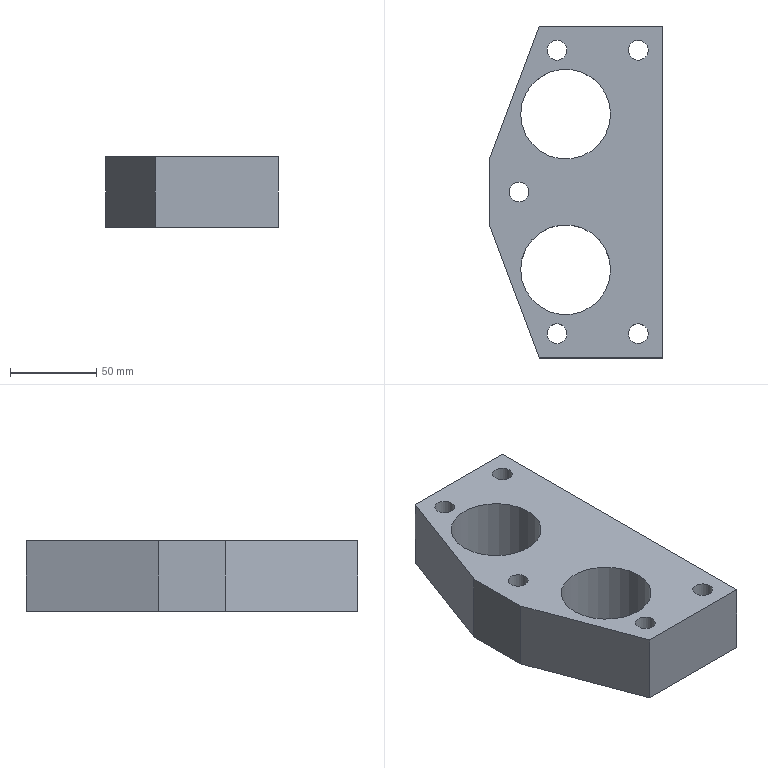Part | NX | features solid 2 | 1 solid | 25 faces | box 100 x 192 x 41 mm | volume 491723 mm3 | plane 13 | cylinder 12 | commonest cylinder face diameters 11.5 x5 18 x5 52 x2
STEP:
#1=CARTESIAN_POINT('',(1356.,82.,60.));
#2=VERTEX_POINT('',#1);
#3=CARTESIAN_POINT('',(1347.,82.,60.));
#4=DIRECTION('',(0.,0.,1.));
#5=DIRECTION('',(1.,0.,0.));
#6=AXIS2_PLACEMENT_3D('',#3,#4,#5);
#7=CIRCLE('',#6,9.);
#8=EDGE_CURVE('',#2,#2,#7,.T.);
#9=ORIENTED_EDGE('',*,*,#8,.T.);
#10=EDGE_LOOP('',(#9));
#11=FACE_BOUND('',#10,.T.);
#12=CARTESIAN_POINT('',(1287.,0.,60.));
#13=VERTEX_POINT('',#12);
#14=CARTESIAN_POINT('',(1278.,0.,60.));
#15=DIRECTION('',(0.,0.,1.));
#16=DIRECTION('',(1.,0.,0.));
#17=AXIS2_PLACEMENT_3D('',#14,#15,#16);
#18=CIRCLE('',#17,9.);
#19=EDGE_CURVE('',#13,#13,#18,.T.);
#20=ORIENTED_EDGE('',*,*,#19,.T.);
#21=EDGE_LOOP('',(#20));
#22=FACE_BOUND('',#21,.T.);
#23=CARTESIAN_POINT('',(1356.,-82.,60.));
#24=VERTEX_POINT('',#23);
#25=CARTESIAN_POINT('',(1347.,-82.,60.));
#26=DIRECTION('',(0.,0.,1.));
#27=DIRECTION('',(1.,0.,0.));
#28=AXIS2_PLACEMENT_3D('',#25,#26,#27);
#29=CIRCLE('',#28,9.);
#30=EDGE_CURVE('',#24,#24,#29,.T.);
#31=ORIENTED_EDGE('',*,*,#30,.T.);
#32=EDGE_LOOP('',(#31));
#33=FACE_BOUND('',#32,.T.);
#34=CARTESIAN_POINT('',(1261.,19.27,60.));
#35=VERTEX_POINT('',#34);
#36=CARTESIAN_POINT('',(1261.,-19.27,60.));
#37=VERTEX_POINT('',#36);
#38=CARTESIAN_POINT('',(1261.,0.,60.));
#39=DIRECTION('',(0.,-1.,0.));
#40=VECTOR('',#39,1000.);
#41=LINE('',#38,#40);
#42=EDGE_CURVE('',#35,#37,#41,.T.);
#43=ORIENTED_EDGE('',*,*,#42,.F.);
#44=CARTESIAN_POINT('',(1289.688,96.,60.));
#45=VERTEX_POINT('',#44);
#46=CARTESIAN_POINT('',(1383.637,347.282,60.));
#47=DIRECTION('',(-0.3502,-0.9367,0.));
#48=VECTOR('',#47,1000.);
#49=LINE('',#46,#48);
#50=EDGE_CURVE('',#45,#35,#49,.T.);
#51=ORIENTED_EDGE('',*,*,#50,.F.);
#52=CARTESIAN_POINT('',(1361.,96.,60.));
#53=VERTEX_POINT('',#52);
#54=CARTESIAN_POINT('',(1390.,96.,60.));
#55=DIRECTION('',(1.,0.,0.));
#56=VECTOR('',#55,1000.);
#57=LINE('',#54,#56);
#58=EDGE_CURVE('',#45,#53,#57,.T.);
#59=ORIENTED_EDGE('',*,*,#58,.T.);
#60=CARTESIAN_POINT('',(1361.,-96.,60.));
#61=VERTEX_POINT('',#60);
#62=CARTESIAN_POINT('',(1361.,0.,60.));
#63=DIRECTION('',(0.,1.,0.));
#64=VECTOR('',#63,1000.);
#65=LINE('',#62,#64);
#66=EDGE_CURVE('',#61,#53,#65,.T.);
#67=ORIENTED_EDGE('',*,*,#66,.F.);
#68=CARTESIAN_POINT('',(1289.688,-96.,60.));
#69=VERTEX_POINT('',#68);
#70=CARTESIAN_POINT('',(1390.,-96.,60.));
#71=DIRECTION('',(1.,0.,0.));
#72=VECTOR('',#71,1000.);
#73=LINE('',#70,#72);
#74=EDGE_CURVE('',#69,#61,#73,.T.);
#75=ORIENTED_EDGE('',*,*,#74,.F.);
#76=CARTESIAN_POINT('',(1383.637,-347.282,60.));
#77=DIRECTION('',(-0.3502,0.9367,0.));
#78=VECTOR('',#77,1000.);
#79=LINE('',#76,#78);
#80=EDGE_CURVE('',#69,#37,#79,.T.);
#81=ORIENTED_EDGE('',*,*,#80,.T.);
#82=EDGE_LOOP('',(#43,#51,#59,#67,#75,#81));
#83=FACE_BOUND('',#82,.T.);
#84=CARTESIAN_POINT('',(1309.,-82.,60.));
#85=VERTEX_POINT('',#84);
#86=CARTESIAN_POINT('',(1300.,-82.,60.));
#87=DIRECTION('',(0.,0.,1.));
#88=DIRECTION('',(1.,0.,0.));
#89=AXIS2_PLACEMENT_3D('',#86,#87,#88);
#90=CIRCLE('',#89,9.);
#91=EDGE_CURVE('',#85,#85,#90,.T.);
#92=ORIENTED_EDGE('',*,*,#91,.T.);
#93=EDGE_LOOP('',(#92));
#94=FACE_BOUND('',#93,.T.);
#95=CARTESIAN_POINT('',(1309.,82.,60.));
#96=VERTEX_POINT('',#95);
#97=CARTESIAN_POINT('',(1300.,82.,60.));
#98=DIRECTION('',(0.,0.,1.));
#99=DIRECTION('',(1.,0.,0.));
#100=AXIS2_PLACEMENT_3D('',#97,#98,#99);
#101=CIRCLE('',#100,9.);
#102=EDGE_CURVE('',#96,#96,#101,.T.);
#103=ORIENTED_EDGE('',*,*,#102,.T.);
#104=EDGE_LOOP('',(#103));
#105=FACE_BOUND('',#104,.T.);
#106=CARTESIAN_POINT('',(1331.,-45.,60.));
#107=VERTEX_POINT('',#106);
#108=CARTESIAN_POINT('',(1305.,-45.,60.));
#109=DIRECTION('',(0.,0.,1.));
#110=DIRECTION('',(1.,0.,0.));
#111=AXIS2_PLACEMENT_3D('',#108,#109,#110);
#112=CIRCLE('',#111,26.);
#113=EDGE_CURVE('',#107,#107,#112,.T.);
#114=ORIENTED_EDGE('',*,*,#113,.T.);
#115=EDGE_LOOP('',(#114));
#116=FACE_BOUND('',#115,.T.);
#117=CARTESIAN_POINT('',(1331.,45.,60.));
#118=VERTEX_POINT('',#117);
#119=CARTESIAN_POINT('',(1305.,45.,60.));
#120=DIRECTION('',(0.,0.,1.));
#121=DIRECTION('',(1.,0.,0.));
#122=AXIS2_PLACEMENT_3D('',#119,#120,#121);
#123=CIRCLE('',#122,26.);
#124=EDGE_CURVE('',#118,#118,#123,.T.);
#125=ORIENTED_EDGE('',*,*,#124,.T.);
#126=EDGE_LOOP('',(#125));
#127=FACE_BOUND('',#126,.T.);
#128=CARTESIAN_POINT('',(2312.5,0.,60.));
#129=DIRECTION('',(0.,0.,1.));
#130=DIRECTION('',(-1.,0.,0.));
#131=AXIS2_PLACEMENT_3D('',#128,#129,#130);
#132=PLANE('',#131);
#133=ADVANCED_FACE('',(#11,#22,#33,#83,#94,#105,#116,#127),#132,.F.);
#134=CARTESIAN_POINT('',(1361.,96.,101.));
#135=VERTEX_POINT('',#134);
#136=CARTESIAN_POINT('',(1361.,-96.,101.));
#137=VERTEX_POINT('',#136);
#138=CARTESIAN_POINT('',(1361.,0.,101.));
#139=DIRECTION('',(0.,-1.,0.));
#140=VECTOR('',#139,1000.);
#141=LINE('',#138,#140);
#142=EDGE_CURVE('',#135,#137,#141,.T.);
#143=ORIENTED_EDGE('',*,*,#142,.F.);
#144=CARTESIAN_POINT('',(1289.688,96.,101.));
#145=VERTEX_POINT('',#144);
#146=CARTESIAN_POINT('',(1390.,96.,101.));
#147=DIRECTION('',(-1.,0.,0.));
#148=VECTOR('',#147,1000.);
#149=LINE('',#146,#148);
#150=EDGE_CURVE('',#135,#145,#149,.T.);
#151=ORIENTED_EDGE('',*,*,#150,.T.);
#152=CARTESIAN_POINT('',(1261.,19.27,101.));
#153=VERTEX_POINT('',#152);
#154=CARTESIAN_POINT('',(1071.365,-487.94,101.));
#155=DIRECTION('',(0.3502,0.9367,0.));
#156=VECTOR('',#155,1000.);
#157=LINE('',#154,#156);
#158=EDGE_CURVE('',#153,#145,#157,.T.);
#159=ORIENTED_EDGE('',*,*,#158,.F.);
#160=CARTESIAN_POINT('',(1261.,-19.27,101.));
#161=VERTEX_POINT('',#160);
#162=CARTESIAN_POINT('',(1261.,0.,101.));
#163=DIRECTION('',(0.,1.,0.));
#164=VECTOR('',#163,1000.);
#165=LINE('',#162,#164);
#166=EDGE_CURVE('',#161,#153,#165,.T.);
#167=ORIENTED_EDGE('',*,*,#166,.F.);
#168=CARTESIAN_POINT('',(1289.688,-96.,101.));
#169=VERTEX_POINT('',#168);
#170=CARTESIAN_POINT('',(1071.365,487.94,101.));
#171=DIRECTION('',(0.3502,-0.9367,0.));
#172=VECTOR('',#171,1000.);
#173=LINE('',#170,#172);
#174=EDGE_CURVE('',#161,#169,#173,.T.);
#175=ORIENTED_EDGE('',*,*,#174,.T.);
#176=CARTESIAN_POINT('',(1390.,-96.,101.));
#177=DIRECTION('',(-1.,0.,0.));
#178=VECTOR('',#177,1000.);
#179=LINE('',#176,#178);
#180=EDGE_CURVE('',#137,#169,#179,.T.);
#181=ORIENTED_EDGE('',*,*,#180,.F.);
#182=EDGE_LOOP('',(#143,#151,#159,#167,#175,#181));
#183=FACE_BOUND('',#182,.T.);
#184=CARTESIAN_POINT('',(1352.75,-82.,101.));
#185=VERTEX_POINT('',#184);
#186=CARTESIAN_POINT('',(1347.,-82.,101.));
#187=DIRECTION('',(0.,0.,1.));
#188=DIRECTION('',(1.,0.,0.));
#189=AXIS2_PLACEMENT_3D('',#186,#187,#188);
#190=CIRCLE('',#189,5.75);
#191=EDGE_CURVE('',#185,#185,#190,.T.);
#192=ORIENTED_EDGE('',*,*,#191,.F.);
#193=EDGE_LOOP('',(#192));
#194=FACE_BOUND('',#193,.T.);
#195=CARTESIAN_POINT('',(1305.75,-82.,101.));
#196=VERTEX_POINT('',#195);
#197=CARTESIAN_POINT('',(1300.,-82.,101.));
#198=DIRECTION('',(0.,0.,1.));
#199=DIRECTION('',(1.,0.,0.));
#200=AXIS2_PLACEMENT_3D('',#197,#198,#199);
#201=CIRCLE('',#200,5.75);
#202=EDGE_CURVE('',#196,#196,#201,.T.);
#203=ORIENTED_EDGE('',*,*,#202,.F.);
#204=EDGE_LOOP('',(#203));
#205=FACE_BOUND('',#204,.T.);
#206=CARTESIAN_POINT('',(1283.75,0.,101.));
#207=VERTEX_POINT('',#206);
#208=CARTESIAN_POINT('',(1278.,0.,101.));
#209=DIRECTION('',(0.,0.,1.));
#210=DIRECTION('',(1.,0.,0.));
#211=AXIS2_PLACEMENT_3D('',#208,#209,#210);
#212=CIRCLE('',#211,5.75);
#213=EDGE_CURVE('',#207,#207,#212,.T.);
#214=ORIENTED_EDGE('',*,*,#213,.F.);
#215=EDGE_LOOP('',(#214));
#216=FACE_BOUND('',#215,.T.);
#217=CARTESIAN_POINT('',(1305.75,82.,101.));
#218=VERTEX_POINT('',#217);
#219=CARTESIAN_POINT('',(1300.,82.,101.));
#220=DIRECTION('',(0.,0.,1.));
#221=DIRECTION('',(1.,0.,0.));
#222=AXIS2_PLACEMENT_3D('',#219,#220,#221);
#223=CIRCLE('',#222,5.75);
#224=EDGE_CURVE('',#218,#218,#223,.T.);
#225=ORIENTED_EDGE('',*,*,#224,.F.);
#226=EDGE_LOOP('',(#225));
#227=FACE_BOUND('',#226,.T.);
#228=CARTESIAN_POINT('',(1352.75,82.,101.));
#229=VERTEX_POINT('',#228);
#230=CARTESIAN_POINT('',(1347.,82.,101.));
#231=DIRECTION('',(0.,0.,1.));
#232=DIRECTION('',(1.,0.,0.));
#233=AXIS2_PLACEMENT_3D('',#230,#231,#232);
#234=CIRCLE('',#233,5.75);
#235=EDGE_CURVE('',#229,#229,#234,.T.);
#236=ORIENTED_EDGE('',*,*,#235,.F.);
#237=EDGE_LOOP('',(#236));
#238=FACE_BOUND('',#237,.T.);
#239=CARTESIAN_POINT('',(1331.,-45.,101.));
#240=VERTEX_POINT('',#239);
#241=CARTESIAN_POINT('',(1305.,-45.,101.));
#242=DIRECTION('',(0.,0.,-1.));
#243=DIRECTION('',(1.,0.,0.));
#244=AXIS2_PLACEMENT_3D('',#241,#242,#243);
#245=CIRCLE('',#244,26.);
#246=EDGE_CURVE('',#240,#240,#245,.T.);
#247=ORIENTED_EDGE('',*,*,#246,.T.);
#248=EDGE_LOOP('',(#247));
#249=FACE_BOUND('',#248,.T.);
#250=CARTESIAN_POINT('',(1331.,45.,101.));
#251=VERTEX_POINT('',#250);
#252=CARTESIAN_POINT('',(1305.,45.,101.));
#253=DIRECTION('',(0.,0.,1.));
#254=DIRECTION('',(1.,0.,0.));
#255=AXIS2_PLACEMENT_3D('',#252,#253,#254);
#256=CIRCLE('',#255,26.);
#257=EDGE_CURVE('',#251,#251,#256,.T.);
#258=ORIENTED_EDGE('',*,*,#257,.F.);
#259=EDGE_LOOP('',(#258));
#260=FACE_BOUND('',#259,.T.);
#261=CARTESIAN_POINT('',(282.5,193.,101.));
#262=DIRECTION('',(0.,0.,1.));
#263=DIRECTION('',(-1.,0.,0.));
#264=AXIS2_PLACEMENT_3D('',#261,#262,#263);
#265=PLANE('',#264);
#266=ADVANCED_FACE('',(#183,#194,#205,#216,#227,#238,#249,#260),#265,.T.);
#267=ORIENTED_EDGE('',*,*,#166,.T.);
#268=CARTESIAN_POINT('',(1261.,19.27,-25.));
#269=DIRECTION('',(0.,0.,1.));
#270=VECTOR('',#269,1000.);
#271=LINE('',#268,#270);
#272=EDGE_CURVE('',#35,#153,#271,.T.);
#273=ORIENTED_EDGE('',*,*,#272,.F.);
#274=ORIENTED_EDGE('',*,*,#42,.T.);
#275=CARTESIAN_POINT('',(1261.,-19.27,-25.));
#276=DIRECTION('',(0.,0.,1.));
#277=VECTOR('',#276,1000.);
#278=LINE('',#275,#277);
#279=EDGE_CURVE('',#37,#161,#278,.T.);
#280=ORIENTED_EDGE('',*,*,#279,.T.);
#281=EDGE_LOOP('',(#267,#273,#274,#280));
#282=FACE_BOUND('',#281,.T.);
#283=CARTESIAN_POINT('',(1261.,0.,-25.));
#284=DIRECTION('',(-1.,0.,0.));
#285=DIRECTION('',(0.,0.,-1.));
#286=AXIS2_PLACEMENT_3D('',#283,#284,#285);
#287=PLANE('',#286);
#288=ADVANCED_FACE('',(#282),#287,.T.);
#289=ORIENTED_EDGE('',*,*,#66,.T.);
#290=CARTESIAN_POINT('',(1361.,96.,0.));
#291=DIRECTION('',(0.,0.,1.));
#292=VECTOR('',#291,1000.);
#293=LINE('',#290,#292);
#294=EDGE_CURVE('',#53,#135,#293,.T.);
#295=ORIENTED_EDGE('',*,*,#294,.T.);
#296=ORIENTED_EDGE('',*,*,#142,.T.);
#297=CARTESIAN_POINT('',(1361.,-96.,0.));
#298=DIRECTION('',(0.,0.,1.));
#299=VECTOR('',#298,1000.);
#300=LINE('',#297,#299);
#301=EDGE_CURVE('',#61,#137,#300,.T.);
#302=ORIENTED_EDGE('',*,*,#301,.F.);
#303=EDGE_LOOP('',(#289,#295,#296,#302));
#304=FACE_BOUND('',#303,.T.);
#305=CARTESIAN_POINT('',(1361.,0.,-25.));
#306=DIRECTION('',(1.,0.,0.));
#307=DIRECTION('',(0.,0.,1.));
#308=AXIS2_PLACEMENT_3D('',#305,#306,#307);
#309=PLANE('',#308);
#310=ADVANCED_FACE('',(#304),#309,.T.);
#311=ORIENTED_EDGE('',*,*,#180,.T.);
#312=CARTESIAN_POINT('',(1289.688,-96.,0.));
#313=DIRECTION('',(0.,0.,-1.));
#314=VECTOR('',#313,1000.);
#315=LINE('',#312,#314);
#316=EDGE_CURVE('',#169,#69,#315,.T.);
#317=ORIENTED_EDGE('',*,*,#316,.T.);
#318=ORIENTED_EDGE('',*,*,#74,.T.);
#319=ORIENTED_EDGE('',*,*,#301,.T.);
#320=EDGE_LOOP('',(#311,#317,#318,#319));
#321=FACE_BOUND('',#320,.T.);
#322=CARTESIAN_POINT('',(1390.,-96.,0.));
#323=DIRECTION('',(0.,-1.,0.));
#324=DIRECTION('',(0.,0.,1.));
#325=AXIS2_PLACEMENT_3D('',#322,#323,#324);
#326=PLANE('',#325);
#327=ADVANCED_FACE('',(#321),#326,.T.);
#328=ORIENTED_EDGE('',*,*,#174,.F.);
#329=ORIENTED_EDGE('',*,*,#279,.F.);
#330=ORIENTED_EDGE('',*,*,#80,.F.);
#331=ORIENTED_EDGE('',*,*,#316,.F.);
#332=EDGE_LOOP('',(#328,#329,#330,#331));
#333=FACE_BOUND('',#332,.T.);
#334=CARTESIAN_POINT('',(1289.418,-95.278,-40.));
#335=DIRECTION('',(-0.9367,-0.3502,0.));
#336=DIRECTION('',(0.3502,-0.9367,0.));
#337=AXIS2_PLACEMENT_3D('',#334,#335,#336);
#338=PLANE('',#337);
#339=ADVANCED_FACE('',(#333),#338,.T.);
#340=ORIENTED_EDGE('',*,*,#150,.F.);
#341=ORIENTED_EDGE('',*,*,#294,.F.);
#342=ORIENTED_EDGE('',*,*,#58,.F.);
#343=CARTESIAN_POINT('',(1289.688,96.,0.));
#344=DIRECTION('',(0.,0.,-1.));
#345=VECTOR('',#344,1000.);
#346=LINE('',#343,#345);
#347=EDGE_CURVE('',#145,#45,#346,.T.);
#348=ORIENTED_EDGE('',*,*,#347,.F.);
#349=EDGE_LOOP('',(#340,#341,#342,#348));
#350=FACE_BOUND('',#349,.T.);
#351=CARTESIAN_POINT('',(1390.,96.,0.));
#352=DIRECTION('',(0.,1.,0.));
#353=DIRECTION('',(0.,0.,1.));
#354=AXIS2_PLACEMENT_3D('',#351,#352,#353);
#355=PLANE('',#354);
#356=ADVANCED_FACE('',(#350),#355,.T.);
#357=ORIENTED_EDGE('',*,*,#158,.T.);
#358=ORIENTED_EDGE('',*,*,#347,.T.);
#359=ORIENTED_EDGE('',*,*,#50,.T.);
#360=ORIENTED_EDGE('',*,*,#272,.T.);
#361=EDGE_LOOP('',(#357,#358,#359,#360));
#362=FACE_BOUND('',#361,.T.);
#363=CARTESIAN_POINT('',(1289.418,95.278,-40.));
#364=DIRECTION('',(-0.9367,0.3502,0.));
#365=DIRECTION('',(0.3502,0.9367,0.));
#366=AXIS2_PLACEMENT_3D('',#363,#364,#365);
#367=PLANE('',#366);
#368=ADVANCED_FACE('',(#362),#367,.T.);
#369=ORIENTED_EDGE('',*,*,#191,.T.);
#370=EDGE_LOOP('',(#369));
#371=FACE_BOUND('',#370,.T.);
#372=CARTESIAN_POINT('',(1352.75,-82.,73.));
#373=VERTEX_POINT('',#372);
#374=CARTESIAN_POINT('',(1347.,-82.,73.));
#375=DIRECTION('',(0.,0.,1.));
#376=DIRECTION('',(1.,0.,0.));
#377=AXIS2_PLACEMENT_3D('',#374,#375,#376);
#378=CIRCLE('',#377,5.75);
#379=EDGE_CURVE('',#373,#373,#378,.T.);
#380=ORIENTED_EDGE('',*,*,#379,.F.);
#381=EDGE_LOOP('',(#380));
#382=FACE_BOUND('',#381,.T.);
#383=CARTESIAN_POINT('',(1347.,-82.,55.));
#384=DIRECTION('',(0.,0.,1.));
#385=DIRECTION('',(-1.,0.,0.));
#386=AXIS2_PLACEMENT_3D('',#383,#384,#385);
#387=CYLINDRICAL_SURFACE('',#386,5.75);
#388=ADVANCED_FACE('',(#371,#382),#387,.F.);
#389=ORIENTED_EDGE('',*,*,#379,.T.);
#390=EDGE_LOOP('',(#389));
#391=FACE_BOUND('',#390,.T.);
#392=CARTESIAN_POINT('',(1356.,-82.,73.));
#393=VERTEX_POINT('',#392);
#394=CARTESIAN_POINT('',(1347.,-82.,73.));
#395=DIRECTION('',(0.,0.,1.));
#396=DIRECTION('',(1.,0.,0.));
#397=AXIS2_PLACEMENT_3D('',#394,#395,#396);
#398=CIRCLE('',#397,9.);
#399=EDGE_CURVE('',#393,#393,#398,.T.);
#400=ORIENTED_EDGE('',*,*,#399,.F.);
#401=EDGE_LOOP('',(#400));
#402=FACE_BOUND('',#401,.T.);
#403=CARTESIAN_POINT('',(1347.,-82.,73.));
#404=DIRECTION('',(0.,0.,1.));
#405=DIRECTION('',(-1.,0.,0.));
#406=AXIS2_PLACEMENT_3D('',#403,#404,#405);
#407=PLANE('',#406);
#408=ADVANCED_FACE('',(#391,#402),#407,.F.);
#409=ORIENTED_EDGE('',*,*,#399,.T.);
#410=EDGE_LOOP('',(#409));
#411=FACE_BOUND('',#410,.T.);
#412=ORIENTED_EDGE('',*,*,#30,.F.);
#413=EDGE_LOOP('',(#412));
#414=FACE_BOUND('',#413,.T.);
#415=CARTESIAN_POINT('',(1347.,-82.,60.));
#416=DIRECTION('',(0.,0.,1.));
#417=DIRECTION('',(-1.,0.,0.));
#418=AXIS2_PLACEMENT_3D('',#415,#416,#417);
#419=CYLINDRICAL_SURFACE('',#418,9.);
#420=ADVANCED_FACE('',(#411,#414),#419,.F.);
#421=ORIENTED_EDGE('',*,*,#202,.T.);
#422=EDGE_LOOP('',(#421));
#423=FACE_BOUND('',#422,.T.);
#424=CARTESIAN_POINT('',(1305.75,-82.,73.));
#425=VERTEX_POINT('',#424);
#426=CARTESIAN_POINT('',(1300.,-82.,73.));
#427=DIRECTION('',(0.,0.,1.));
#428=DIRECTION('',(1.,0.,0.));
#429=AXIS2_PLACEMENT_3D('',#426,#427,#428);
#430=CIRCLE('',#429,5.75);
#431=EDGE_CURVE('',#425,#425,#430,.T.);
#432=ORIENTED_EDGE('',*,*,#431,.F.);
#433=EDGE_LOOP('',(#432));
#434=FACE_BOUND('',#433,.T.);
#435=CARTESIAN_POINT('',(1300.,-82.,55.));
#436=DIRECTION('',(0.,0.,1.));
#437=DIRECTION('',(-1.,0.,0.));
#438=AXIS2_PLACEMENT_3D('',#435,#436,#437);
#439=CYLINDRICAL_SURFACE('',#438,5.75);
#440=ADVANCED_FACE('',(#423,#434),#439,.F.);
#441=ORIENTED_EDGE('',*,*,#431,.T.);
#442=EDGE_LOOP('',(#441));
#443=FACE_BOUND('',#442,.T.);
#444=CARTESIAN_POINT('',(1309.,-82.,73.));
#445=VERTEX_POINT('',#444);
#446=CARTESIAN_POINT('',(1300.,-82.,73.));
#447=DIRECTION('',(0.,0.,1.));
#448=DIRECTION('',(1.,0.,0.));
#449=AXIS2_PLACEMENT_3D('',#446,#447,#448);
#450=CIRCLE('',#449,9.);
#451=EDGE_CURVE('',#445,#445,#450,.T.);
#452=ORIENTED_EDGE('',*,*,#451,.F.);
#453=EDGE_LOOP('',(#452));
#454=FACE_BOUND('',#453,.T.);
#455=CARTESIAN_POINT('',(1300.,-82.,73.));
#456=DIRECTION('',(0.,0.,1.));
#457=DIRECTION('',(-1.,0.,0.));
#458=AXIS2_PLACEMENT_3D('',#455,#456,#457);
#459=PLANE('',#458);
#460=ADVANCED_FACE('',(#443,#454),#459,.F.);
#461=ORIENTED_EDGE('',*,*,#451,.T.);
#462=EDGE_LOOP('',(#461));
#463=FACE_BOUND('',#462,.T.);
#464=ORIENTED_EDGE('',*,*,#91,.F.);
#465=EDGE_LOOP('',(#464));
#466=FACE_BOUND('',#465,.T.);
#467=CARTESIAN_POINT('',(1300.,-82.,60.));
#468=DIRECTION('',(0.,0.,1.));
#469=DIRECTION('',(-1.,0.,0.));
#470=AXIS2_PLACEMENT_3D('',#467,#468,#469);
#471=CYLINDRICAL_SURFACE('',#470,9.);
#472=ADVANCED_FACE('',(#463,#466),#471,.F.);
#473=ORIENTED_EDGE('',*,*,#213,.T.);
#474=EDGE_LOOP('',(#473));
#475=FACE_BOUND('',#474,.T.);
#476=CARTESIAN_POINT('',(1283.75,0.,73.));
#477=VERTEX_POINT('',#476);
#478=CARTESIAN_POINT('',(1278.,0.,73.));
#479=DIRECTION('',(0.,0.,1.));
#480=DIRECTION('',(1.,0.,0.));
#481=AXIS2_PLACEMENT_3D('',#478,#479,#480);
#482=CIRCLE('',#481,5.75);
#483=EDGE_CURVE('',#477,#477,#482,.T.);
#484=ORIENTED_EDGE('',*,*,#483,.F.);
#485=EDGE_LOOP('',(#484));
#486=FACE_BOUND('',#485,.T.);
#487=CARTESIAN_POINT('',(1278.,0.,55.));
#488=DIRECTION('',(0.,0.,1.));
#489=DIRECTION('',(-1.,0.,0.));
#490=AXIS2_PLACEMENT_3D('',#487,#488,#489);
#491=CYLINDRICAL_SURFACE('',#490,5.75);
#492=ADVANCED_FACE('',(#475,#486),#491,.F.);
#493=ORIENTED_EDGE('',*,*,#483,.T.);
#494=EDGE_LOOP('',(#493));
#495=FACE_BOUND('',#494,.T.);
#496=CARTESIAN_POINT('',(1287.,0.,73.));
#497=VERTEX_POINT('',#496);
#498=CARTESIAN_POINT('',(1278.,0.,73.));
#499=DIRECTION('',(0.,0.,1.));
#500=DIRECTION('',(1.,0.,0.));
#501=AXIS2_PLACEMENT_3D('',#498,#499,#500);
#502=CIRCLE('',#501,9.);
#503=EDGE_CURVE('',#497,#497,#502,.T.);
#504=ORIENTED_EDGE('',*,*,#503,.F.);
#505=EDGE_LOOP('',(#504));
#506=FACE_BOUND('',#505,.T.);
#507=CARTESIAN_POINT('',(1278.,0.,73.));
#508=DIRECTION('',(0.,0.,1.));
#509=DIRECTION('',(-1.,0.,0.));
#510=AXIS2_PLACEMENT_3D('',#507,#508,#509);
#511=PLANE('',#510);
#512=ADVANCED_FACE('',(#495,#506),#511,.F.);
#513=ORIENTED_EDGE('',*,*,#503,.T.);
#514=EDGE_LOOP('',(#513));
#515=FACE_BOUND('',#514,.T.);
#516=ORIENTED_EDGE('',*,*,#19,.F.);
#517=EDGE_LOOP('',(#516));
#518=FACE_BOUND('',#517,.T.);
#519=CARTESIAN_POINT('',(1278.,0.,60.));
#520=DIRECTION('',(0.,0.,1.));
#521=DIRECTION('',(-1.,0.,0.));
#522=AXIS2_PLACEMENT_3D('',#519,#520,#521);
#523=CYLINDRICAL_SURFACE('',#522,9.);
#524=ADVANCED_FACE('',(#515,#518),#523,.F.);
#525=ORIENTED_EDGE('',*,*,#224,.T.);
#526=EDGE_LOOP('',(#525));
#527=FACE_BOUND('',#526,.T.);
#528=CARTESIAN_POINT('',(1305.75,82.,73.));
#529=VERTEX_POINT('',#528);
#530=CARTESIAN_POINT('',(1300.,82.,73.));
#531=DIRECTION('',(0.,0.,1.));
#532=DIRECTION('',(1.,0.,0.));
#533=AXIS2_PLACEMENT_3D('',#530,#531,#532);
#534=CIRCLE('',#533,5.75);
#535=EDGE_CURVE('',#529,#529,#534,.T.);
#536=ORIENTED_EDGE('',*,*,#535,.F.);
#537=EDGE_LOOP('',(#536));
#538=FACE_BOUND('',#537,.T.);
#539=CARTESIAN_POINT('',(1300.,82.,55.));
#540=DIRECTION('',(0.,0.,1.));
#541=DIRECTION('',(-1.,0.,0.));
#542=AXIS2_PLACEMENT_3D('',#539,#540,#541);
#543=CYLINDRICAL_SURFACE('',#542,5.75);
#544=ADVANCED_FACE('',(#527,#538),#543,.F.);
#545=ORIENTED_EDGE('',*,*,#535,.T.);
#546=EDGE_LOOP('',(#545));
#547=FACE_BOUND('',#546,.T.);
#548=CARTESIAN_POINT('',(1309.,82.,73.));
#549=VERTEX_POINT('',#548);
#550=CARTESIAN_POINT('',(1300.,82.,73.));
#551=DIRECTION('',(0.,0.,1.));
#552=DIRECTION('',(1.,0.,0.));
#553=AXIS2_PLACEMENT_3D('',#550,#551,#552);
#554=CIRCLE('',#553,9.);
#555=EDGE_CURVE('',#549,#549,#554,.T.);
#556=ORIENTED_EDGE('',*,*,#555,.F.);
#557=EDGE_LOOP('',(#556));
#558=FACE_BOUND('',#557,.T.);
#559=CARTESIAN_POINT('',(1300.,82.,73.));
#560=DIRECTION('',(0.,0.,1.));
#561=DIRECTION('',(-1.,0.,0.));
#562=AXIS2_PLACEMENT_3D('',#559,#560,#561);
#563=PLANE('',#562);
#564=ADVANCED_FACE('',(#547,#558),#563,.F.);
#565=ORIENTED_EDGE('',*,*,#555,.T.);
#566=EDGE_LOOP('',(#565));
#567=FACE_BOUND('',#566,.T.);
#568=ORIENTED_EDGE('',*,*,#102,.F.);
#569=EDGE_LOOP('',(#568));
#570=FACE_BOUND('',#569,.T.);
#571=CARTESIAN_POINT('',(1300.,82.,60.));
#572=DIRECTION('',(0.,0.,1.));
#573=DIRECTION('',(-1.,0.,0.));
#574=AXIS2_PLACEMENT_3D('',#571,#572,#573);
#575=CYLINDRICAL_SURFACE('',#574,9.);
#576=ADVANCED_FACE('',(#567,#570),#575,.F.);
#577=ORIENTED_EDGE('',*,*,#235,.T.);
#578=EDGE_LOOP('',(#577));
#579=FACE_BOUND('',#578,.T.);
#580=CARTESIAN_POINT('',(1352.75,82.,73.));
#581=VERTEX_POINT('',#580);
#582=CARTESIAN_POINT('',(1347.,82.,73.));
#583=DIRECTION('',(0.,0.,1.));
#584=DIRECTION('',(1.,0.,0.));
#585=AXIS2_PLACEMENT_3D('',#582,#583,#584);
#586=CIRCLE('',#585,5.75);
#587=EDGE_CURVE('',#581,#581,#586,.T.);
#588=ORIENTED_EDGE('',*,*,#587,.F.);
#589=EDGE_LOOP('',(#588));
#590=FACE_BOUND('',#589,.T.);
#591=CARTESIAN_POINT('',(1347.,82.,55.));
#592=DIRECTION('',(0.,0.,1.));
#593=DIRECTION('',(-1.,0.,0.));
#594=AXIS2_PLACEMENT_3D('',#591,#592,#593);
#595=CYLINDRICAL_SURFACE('',#594,5.75);
#596=ADVANCED_FACE('',(#579,#590),#595,.F.);
#597=ORIENTED_EDGE('',*,*,#587,.T.);
#598=EDGE_LOOP('',(#597));
#599=FACE_BOUND('',#598,.T.);
#600=CARTESIAN_POINT('',(1356.,82.,73.));
#601=VERTEX_POINT('',#600);
#602=CARTESIAN_POINT('',(1347.,82.,73.));
#603=DIRECTION('',(0.,0.,1.));
#604=DIRECTION('',(1.,0.,0.));
#605=AXIS2_PLACEMENT_3D('',#602,#603,#604);
#606=CIRCLE('',#605,9.);
#607=EDGE_CURVE('',#601,#601,#606,.T.);
#608=ORIENTED_EDGE('',*,*,#607,.F.);
#609=EDGE_LOOP('',(#608));
#610=FACE_BOUND('',#609,.T.);
#611=CARTESIAN_POINT('',(1347.,82.,73.));
#612=DIRECTION('',(0.,0.,1.));
#613=DIRECTION('',(-1.,0.,0.));
#614=AXIS2_PLACEMENT_3D('',#611,#612,#613);
#615=PLANE('',#614);
#616=ADVANCED_FACE('',(#599,#610),#615,.F.);
#617=ORIENTED_EDGE('',*,*,#607,.T.);
#618=EDGE_LOOP('',(#617));
#619=FACE_BOUND('',#618,.T.);
#620=ORIENTED_EDGE('',*,*,#8,.F.);
#621=EDGE_LOOP('',(#620));
#622=FACE_BOUND('',#621,.T.);
#623=CARTESIAN_POINT('',(1347.,82.,60.));
#624=DIRECTION('',(0.,0.,1.));
#625=DIRECTION('',(-1.,0.,0.));
#626=AXIS2_PLACEMENT_3D('',#623,#624,#625);
#627=CYLINDRICAL_SURFACE('',#626,9.);
#628=ADVANCED_FACE('',(#619,#622),#627,.F.);
#629=ORIENTED_EDGE('',*,*,#113,.F.);
#630=EDGE_LOOP('',(#629));
#631=FACE_BOUND('',#630,.T.);
#632=ORIENTED_EDGE('',*,*,#246,.F.);
#633=EDGE_LOOP('',(#632));
#634=FACE_BOUND('',#633,.T.);
#635=CARTESIAN_POINT('',(1305.,-45.,-181.));
#636=DIRECTION('',(0.,0.,1.));
#637=DIRECTION('',(-1.,0.,0.));
#638=AXIS2_PLACEMENT_3D('',#635,#636,#637);
#639=CYLINDRICAL_SURFACE('',#638,26.);
#640=ADVANCED_FACE('',(#631,#634),#639,.F.);
#641=ORIENTED_EDGE('',*,*,#124,.F.);
#642=EDGE_LOOP('',(#641));
#643=FACE_BOUND('',#642,.T.);
#644=ORIENTED_EDGE('',*,*,#257,.T.);
#645=EDGE_LOOP('',(#644));
#646=FACE_BOUND('',#645,.T.);
#647=CARTESIAN_POINT('',(1305.,45.,-181.));
#648=DIRECTION('',(0.,0.,1.));
#649=DIRECTION('',(-1.,0.,0.));
#650=AXIS2_PLACEMENT_3D('',#647,#648,#649);
#651=CYLINDRICAL_SURFACE('',#650,26.);
#652=ADVANCED_FACE('',(#643,#646),#651,.F.);
#653=CLOSED_SHELL('',(#133,#266,#288,#310,#327,#339,#356,#368,#388,#408,#420,#440,#460,#472,#492,#512,#524,#544,#564,#576,#596,#616,#628,#640,#652));
#654=MANIFOLD_SOLID_BREP('',#653);
#655=(LENGTH_UNIT()NAMED_UNIT(*)SI_UNIT(.MILLI.,.METRE.));
#656=UNCERTAINTY_MEASURE_WITH_UNIT(LENGTH_MEASURE(0.00001),#655,'','');
#657=(NAMED_UNIT(*)PLANE_ANGLE_UNIT()SI_UNIT($,.RADIAN.));
#658=(NAMED_UNIT(*)SI_UNIT($,.STERADIAN.)SOLID_ANGLE_UNIT());
#659=(GEOMETRIC_REPRESENTATION_CONTEXT(3)GLOBAL_UNCERTAINTY_ASSIGNED_CONTEXT((#656))GLOBAL_UNIT_ASSIGNED_CONTEXT((#655,#657,#658))REPRESENTATION_CONTEXT('',''));
#660=ADVANCED_BREP_SHAPE_REPRESENTATION('',(#654),#659);